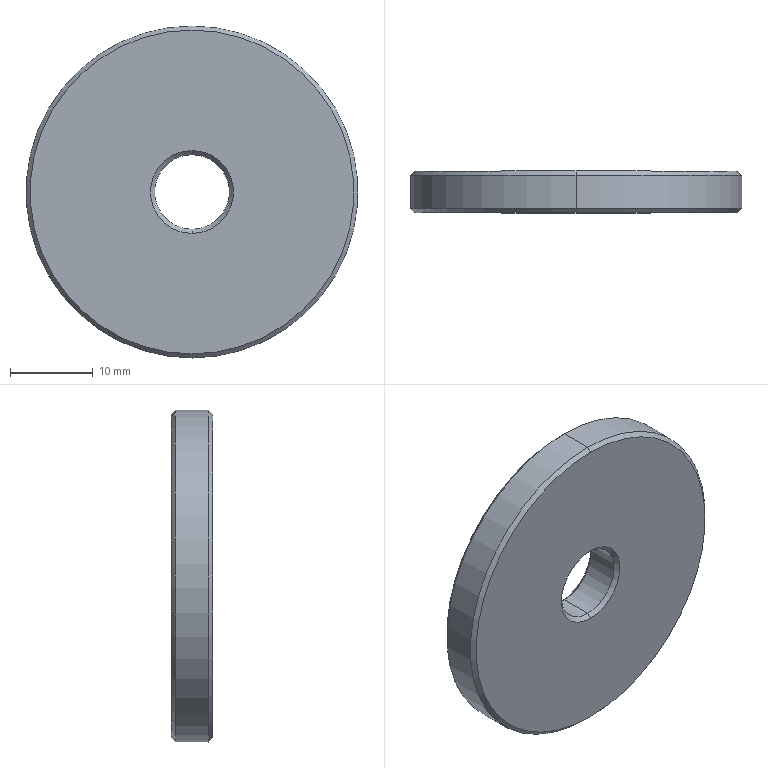Part | SolidWorks | features BaseBody 1 | 1 solid | 14 faces | box 40 x 5 x 40 mm | volume 5927 mm3 | cone 8 | cylinder 4 | plane 2 | commonest cylinder face diameters 9 x2 40 x2
STEP:
#1=CARTESIAN_POINT('',(0.,4.5,-4.5));
#2=VERTEX_POINT('',#1);
#3=CARTESIAN_POINT('',(0.,4.5,4.5));
#4=VERTEX_POINT('',#3);
#5=CARTESIAN_POINT('',(0.,4.5,0.));
#6=DIRECTION('',(0.,1.,0.));
#7=DIRECTION('',(0.,0.,-1.));
#8=AXIS2_PLACEMENT_3D('',#5,#6,#7);
#9=CIRCLE('',#8,4.5);
#10=EDGE_CURVE('',#2,#4,#9,.T.);
#11=ORIENTED_EDGE('',*,*,#10,.F.);
#12=CARTESIAN_POINT('',(0.,5.,-5.));
#13=VERTEX_POINT('',#12);
#14=CARTESIAN_POINT('',(0.,5.,-5.));
#15=DIRECTION('',(0.,0.7071,-0.7071));
#16=VECTOR('',#15,1000.);
#17=LINE('',#14,#16);
#18=EDGE_CURVE('',#2,#13,#17,.T.);
#19=ORIENTED_EDGE('',*,*,#18,.T.);
#20=CARTESIAN_POINT('',(0.,5.,5.));
#21=VERTEX_POINT('',#20);
#22=CARTESIAN_POINT('',(0.,5.,0.));
#23=DIRECTION('',(0.,-1.,0.));
#24=DIRECTION('',(0.,0.,1.));
#25=AXIS2_PLACEMENT_3D('',#22,#23,#24);
#26=CIRCLE('',#25,5.);
#27=EDGE_CURVE('',#21,#13,#26,.T.);
#28=ORIENTED_EDGE('',*,*,#27,.F.);
#29=CARTESIAN_POINT('',(0.,5.,5.));
#30=DIRECTION('',(0.,0.7071,0.7071));
#31=VECTOR('',#30,1000.);
#32=LINE('',#29,#31);
#33=EDGE_CURVE('',#4,#21,#32,.T.);
#34=ORIENTED_EDGE('',*,*,#33,.F.);
#35=EDGE_LOOP('',(#11,#19,#28,#34));
#36=FACE_OUTER_BOUND('',#35,.T.);
#37=CARTESIAN_POINT('',(0.,5.,0.));
#38=DIRECTION('',(0.,1.,0.));
#39=DIRECTION('',(0.,0.,1.));
#40=AXIS2_PLACEMENT_3D('',#37,#38,#39);
#41=CONICAL_SURFACE('',#40,5.,0.7854);
#42=ADVANCED_FACE('',(#36),#41,.F.);
#43=CARTESIAN_POINT('',(0.,5.,19.5));
#44=VERTEX_POINT('',#43);
#45=CARTESIAN_POINT('',(0.,5.,-19.5));
#46=VERTEX_POINT('',#45);
#47=CARTESIAN_POINT('',(0.,5.,0.));
#48=DIRECTION('',(0.,1.,0.));
#49=DIRECTION('',(0.,0.,-1.));
#50=AXIS2_PLACEMENT_3D('',#47,#48,#49);
#51=CIRCLE('',#50,19.5);
#52=EDGE_CURVE('',#44,#46,#51,.T.);
#53=ORIENTED_EDGE('',*,*,#52,.F.);
#54=CARTESIAN_POINT('',(0.,4.5,20.));
#55=VERTEX_POINT('',#54);
#56=CARTESIAN_POINT('',(0.,4.5,20.));
#57=DIRECTION('',(0.,-0.7071,0.7071));
#58=VECTOR('',#57,1000.);
#59=LINE('',#56,#58);
#60=EDGE_CURVE('',#44,#55,#59,.T.);
#61=ORIENTED_EDGE('',*,*,#60,.T.);
#62=CARTESIAN_POINT('',(0.,4.5,-20.));
#63=VERTEX_POINT('',#62);
#64=CARTESIAN_POINT('',(0.,4.5,0.));
#65=DIRECTION('',(0.,1.,0.));
#66=DIRECTION('',(0.,0.,-1.));
#67=AXIS2_PLACEMENT_3D('',#64,#65,#66);
#68=CIRCLE('',#67,20.);
#69=EDGE_CURVE('',#55,#63,#68,.T.);
#70=ORIENTED_EDGE('',*,*,#69,.T.);
#71=CARTESIAN_POINT('',(0.,4.5,-20.));
#72=DIRECTION('',(0.,-0.7071,-0.7071));
#73=VECTOR('',#72,1000.);
#74=LINE('',#71,#73);
#75=EDGE_CURVE('',#46,#63,#74,.T.);
#76=ORIENTED_EDGE('',*,*,#75,.F.);
#77=EDGE_LOOP('',(#53,#61,#70,#76));
#78=FACE_OUTER_BOUND('',#77,.T.);
#79=CARTESIAN_POINT('',(0.,4.5,0.));
#80=DIRECTION('',(0.,-1.,0.));
#81=DIRECTION('',(0.,0.,-1.));
#82=AXIS2_PLACEMENT_3D('',#79,#80,#81);
#83=CONICAL_SURFACE('',#82,20.,0.7854);
#84=ADVANCED_FACE('',(#78),#83,.T.);
#85=CARTESIAN_POINT('',(0.,0.5,-4.5));
#86=VERTEX_POINT('',#85);
#87=CARTESIAN_POINT('',(0.,0.5,4.5));
#88=VERTEX_POINT('',#87);
#89=CARTESIAN_POINT('',(0.,0.5,0.));
#90=DIRECTION('',(0.,1.,0.));
#91=DIRECTION('',(0.,0.,1.));
#92=AXIS2_PLACEMENT_3D('',#89,#90,#91);
#93=CIRCLE('',#92,4.5);
#94=EDGE_CURVE('',#86,#88,#93,.T.);
#95=ORIENTED_EDGE('',*,*,#94,.F.);
#96=CARTESIAN_POINT('',(0.,0.,-4.5));
#97=DIRECTION('',(0.,1.,0.));
#98=VECTOR('',#97,1000.);
#99=LINE('',#96,#98);
#100=EDGE_CURVE('',#86,#2,#99,.T.);
#101=ORIENTED_EDGE('',*,*,#100,.T.);
#102=ORIENTED_EDGE('',*,*,#10,.T.);
#103=CARTESIAN_POINT('',(0.,0.,4.5));
#104=DIRECTION('',(0.,1.,0.));
#105=VECTOR('',#104,1000.);
#106=LINE('',#103,#105);
#107=EDGE_CURVE('',#88,#4,#106,.T.);
#108=ORIENTED_EDGE('',*,*,#107,.F.);
#109=EDGE_LOOP('',(#95,#101,#102,#108));
#110=FACE_OUTER_BOUND('',#109,.T.);
#111=CARTESIAN_POINT('',(0.,0.,0.));
#112=DIRECTION('',(0.,1.,0.));
#113=DIRECTION('',(0.,0.,1.));
#114=AXIS2_PLACEMENT_3D('',#111,#112,#113);
#115=CYLINDRICAL_SURFACE('',#114,4.5);
#116=ADVANCED_FACE('',(#110),#115,.F.);
#117=CARTESIAN_POINT('',(0.,0.5,20.));
#118=VERTEX_POINT('',#117);
#119=CARTESIAN_POINT('',(0.,0.5,-20.));
#120=VERTEX_POINT('',#119);
#121=CARTESIAN_POINT('',(0.,0.5,0.));
#122=DIRECTION('',(0.,1.,0.));
#123=DIRECTION('',(0.,0.,1.));
#124=AXIS2_PLACEMENT_3D('',#121,#122,#123);
#125=CIRCLE('',#124,20.);
#126=EDGE_CURVE('',#118,#120,#125,.T.);
#127=ORIENTED_EDGE('',*,*,#126,.T.);
#128=CARTESIAN_POINT('',(0.,0.,-20.));
#129=DIRECTION('',(0.,1.,0.));
#130=VECTOR('',#129,1000.);
#131=LINE('',#128,#130);
#132=EDGE_CURVE('',#120,#63,#131,.T.);
#133=ORIENTED_EDGE('',*,*,#132,.T.);
#134=ORIENTED_EDGE('',*,*,#69,.F.);
#135=CARTESIAN_POINT('',(0.,0.,20.));
#136=DIRECTION('',(0.,1.,0.));
#137=VECTOR('',#136,1000.);
#138=LINE('',#135,#137);
#139=EDGE_CURVE('',#118,#55,#138,.T.);
#140=ORIENTED_EDGE('',*,*,#139,.F.);
#141=EDGE_LOOP('',(#127,#133,#134,#140));
#142=FACE_OUTER_BOUND('',#141,.T.);
#143=CARTESIAN_POINT('',(0.,0.,0.));
#144=DIRECTION('',(0.,1.,0.));
#145=DIRECTION('',(0.,0.,1.));
#146=AXIS2_PLACEMENT_3D('',#143,#144,#145);
#147=CYLINDRICAL_SURFACE('',#146,20.);
#148=ADVANCED_FACE('',(#142),#147,.T.);
#149=ORIENTED_EDGE('',*,*,#94,.T.);
#150=CARTESIAN_POINT('',(0.,0.,5.));
#151=VERTEX_POINT('',#150);
#152=CARTESIAN_POINT('',(0.,0.,5.));
#153=DIRECTION('',(0.,-0.7071,0.7071));
#154=VECTOR('',#153,1000.);
#155=LINE('',#152,#154);
#156=EDGE_CURVE('',#88,#151,#155,.T.);
#157=ORIENTED_EDGE('',*,*,#156,.T.);
#158=CARTESIAN_POINT('',(0.,0.,-5.));
#159=VERTEX_POINT('',#158);
#160=CARTESIAN_POINT('',(0.,0.,0.));
#161=DIRECTION('',(0.,1.,0.));
#162=DIRECTION('',(0.,0.,-1.));
#163=AXIS2_PLACEMENT_3D('',#160,#161,#162);
#164=CIRCLE('',#163,5.);
#165=EDGE_CURVE('',#159,#151,#164,.T.);
#166=ORIENTED_EDGE('',*,*,#165,.F.);
#167=CARTESIAN_POINT('',(0.,0.,-5.));
#168=DIRECTION('',(0.,-0.7071,-0.7071));
#169=VECTOR('',#168,1000.);
#170=LINE('',#167,#169);
#171=EDGE_CURVE('',#86,#159,#170,.T.);
#172=ORIENTED_EDGE('',*,*,#171,.F.);
#173=EDGE_LOOP('',(#149,#157,#166,#172));
#174=FACE_OUTER_BOUND('',#173,.T.);
#175=CARTESIAN_POINT('',(0.,0.,0.));
#176=DIRECTION('',(0.,-1.,0.));
#177=DIRECTION('',(0.,0.,-1.));
#178=AXIS2_PLACEMENT_3D('',#175,#176,#177);
#179=CONICAL_SURFACE('',#178,5.,0.7854);
#180=ADVANCED_FACE('',(#174),#179,.F.);
#181=CARTESIAN_POINT('',(0.,0.,19.5));
#182=VERTEX_POINT('',#181);
#183=CARTESIAN_POINT('',(0.,0.,-19.5));
#184=VERTEX_POINT('',#183);
#185=CARTESIAN_POINT('',(0.,0.,0.));
#186=DIRECTION('',(0.,1.,0.));
#187=DIRECTION('',(0.,0.,1.));
#188=AXIS2_PLACEMENT_3D('',#185,#186,#187);
#189=CIRCLE('',#188,19.5);
#190=EDGE_CURVE('',#182,#184,#189,.T.);
#191=ORIENTED_EDGE('',*,*,#190,.T.);
#192=CARTESIAN_POINT('',(0.,0.5,-20.));
#193=DIRECTION('',(0.,0.7071,-0.7071));
#194=VECTOR('',#193,1000.);
#195=LINE('',#192,#194);
#196=EDGE_CURVE('',#184,#120,#195,.T.);
#197=ORIENTED_EDGE('',*,*,#196,.T.);
#198=ORIENTED_EDGE('',*,*,#126,.F.);
#199=CARTESIAN_POINT('',(0.,0.5,20.));
#200=DIRECTION('',(0.,0.7071,0.7071));
#201=VECTOR('',#200,1000.);
#202=LINE('',#199,#201);
#203=EDGE_CURVE('',#182,#118,#202,.T.);
#204=ORIENTED_EDGE('',*,*,#203,.F.);
#205=EDGE_LOOP('',(#191,#197,#198,#204));
#206=FACE_OUTER_BOUND('',#205,.T.);
#207=CARTESIAN_POINT('',(0.,0.5,0.));
#208=DIRECTION('',(0.,1.,0.));
#209=DIRECTION('',(0.,0.,1.));
#210=AXIS2_PLACEMENT_3D('',#207,#208,#209);
#211=CONICAL_SURFACE('',#210,20.,0.7854);
#212=ADVANCED_FACE('',(#206),#211,.T.);
#213=ORIENTED_EDGE('',*,*,#27,.T.);
#214=CARTESIAN_POINT('',(0.,5.,0.));
#215=DIRECTION('',(0.,-1.,0.));
#216=DIRECTION('',(0.,0.,1.));
#217=AXIS2_PLACEMENT_3D('',#214,#215,#216);
#218=CIRCLE('',#217,5.);
#219=EDGE_CURVE('',#13,#21,#218,.T.);
#220=ORIENTED_EDGE('',*,*,#219,.T.);
#221=EDGE_LOOP('',(#213,#220));
#222=FACE_BOUND('',#221,.T.);
#223=CARTESIAN_POINT('',(0.,5.,0.));
#224=DIRECTION('',(0.,1.,0.));
#225=DIRECTION('',(0.,0.,-1.));
#226=AXIS2_PLACEMENT_3D('',#223,#224,#225);
#227=CIRCLE('',#226,19.5);
#228=EDGE_CURVE('',#46,#44,#227,.T.);
#229=ORIENTED_EDGE('',*,*,#228,.T.);
#230=ORIENTED_EDGE('',*,*,#52,.T.);
#231=EDGE_LOOP('',(#229,#230));
#232=FACE_OUTER_BOUND('',#231,.T.);
#233=CARTESIAN_POINT('',(0.,5.,0.));
#234=DIRECTION('',(0.,1.,0.));
#235=DIRECTION('',(0.,0.,1.));
#236=AXIS2_PLACEMENT_3D('',#233,#234,#235);
#237=PLANE('',#236);
#238=ADVANCED_FACE('',(#222,#232),#237,.T.);
#239=ORIENTED_EDGE('',*,*,#18,.F.);
#240=CARTESIAN_POINT('',(0.,4.5,0.));
#241=DIRECTION('',(0.,1.,0.));
#242=DIRECTION('',(0.,0.,-1.));
#243=AXIS2_PLACEMENT_3D('',#240,#241,#242);
#244=CIRCLE('',#243,4.5);
#245=EDGE_CURVE('',#4,#2,#244,.T.);
#246=ORIENTED_EDGE('',*,*,#245,.F.);
#247=ORIENTED_EDGE('',*,*,#33,.T.);
#248=ORIENTED_EDGE('',*,*,#219,.F.);
#249=EDGE_LOOP('',(#239,#246,#247,#248));
#250=FACE_OUTER_BOUND('',#249,.T.);
#251=CARTESIAN_POINT('',(0.,5.,0.));
#252=DIRECTION('',(0.,1.,0.));
#253=DIRECTION('',(0.,0.,1.));
#254=AXIS2_PLACEMENT_3D('',#251,#252,#253);
#255=CONICAL_SURFACE('',#254,5.,0.7854);
#256=ADVANCED_FACE('',(#250),#255,.F.);
#257=ORIENTED_EDGE('',*,*,#60,.F.);
#258=ORIENTED_EDGE('',*,*,#228,.F.);
#259=ORIENTED_EDGE('',*,*,#75,.T.);
#260=CARTESIAN_POINT('',(0.,4.5,0.));
#261=DIRECTION('',(0.,1.,0.));
#262=DIRECTION('',(0.,0.,-1.));
#263=AXIS2_PLACEMENT_3D('',#260,#261,#262);
#264=CIRCLE('',#263,20.);
#265=EDGE_CURVE('',#63,#55,#264,.T.);
#266=ORIENTED_EDGE('',*,*,#265,.T.);
#267=EDGE_LOOP('',(#257,#258,#259,#266));
#268=FACE_OUTER_BOUND('',#267,.T.);
#269=CARTESIAN_POINT('',(0.,4.5,0.));
#270=DIRECTION('',(0.,-1.,0.));
#271=DIRECTION('',(0.,0.,-1.));
#272=AXIS2_PLACEMENT_3D('',#269,#270,#271);
#273=CONICAL_SURFACE('',#272,20.,0.7854);
#274=ADVANCED_FACE('',(#268),#273,.T.);
#275=ORIENTED_EDGE('',*,*,#100,.F.);
#276=CARTESIAN_POINT('',(0.,0.5,0.));
#277=DIRECTION('',(0.,1.,0.));
#278=DIRECTION('',(0.,0.,1.));
#279=AXIS2_PLACEMENT_3D('',#276,#277,#278);
#280=CIRCLE('',#279,4.5);
#281=EDGE_CURVE('',#88,#86,#280,.T.);
#282=ORIENTED_EDGE('',*,*,#281,.F.);
#283=ORIENTED_EDGE('',*,*,#107,.T.);
#284=ORIENTED_EDGE('',*,*,#245,.T.);
#285=EDGE_LOOP('',(#275,#282,#283,#284));
#286=FACE_OUTER_BOUND('',#285,.T.);
#287=CARTESIAN_POINT('',(0.,0.,0.));
#288=DIRECTION('',(0.,1.,0.));
#289=DIRECTION('',(0.,0.,1.));
#290=AXIS2_PLACEMENT_3D('',#287,#288,#289);
#291=CYLINDRICAL_SURFACE('',#290,4.5);
#292=ADVANCED_FACE('',(#286),#291,.F.);
#293=ORIENTED_EDGE('',*,*,#132,.F.);
#294=CARTESIAN_POINT('',(0.,0.5,0.));
#295=DIRECTION('',(0.,1.,0.));
#296=DIRECTION('',(0.,0.,1.));
#297=AXIS2_PLACEMENT_3D('',#294,#295,#296);
#298=CIRCLE('',#297,20.);
#299=EDGE_CURVE('',#120,#118,#298,.T.);
#300=ORIENTED_EDGE('',*,*,#299,.T.);
#301=ORIENTED_EDGE('',*,*,#139,.T.);
#302=ORIENTED_EDGE('',*,*,#265,.F.);
#303=EDGE_LOOP('',(#293,#300,#301,#302));
#304=FACE_OUTER_BOUND('',#303,.T.);
#305=CARTESIAN_POINT('',(0.,0.,0.));
#306=DIRECTION('',(0.,1.,0.));
#307=DIRECTION('',(0.,0.,1.));
#308=AXIS2_PLACEMENT_3D('',#305,#306,#307);
#309=CYLINDRICAL_SURFACE('',#308,20.);
#310=ADVANCED_FACE('',(#304),#309,.T.);
#311=ORIENTED_EDGE('',*,*,#156,.F.);
#312=ORIENTED_EDGE('',*,*,#281,.T.);
#313=ORIENTED_EDGE('',*,*,#171,.T.);
#314=CARTESIAN_POINT('',(0.,0.,0.));
#315=DIRECTION('',(0.,1.,0.));
#316=DIRECTION('',(0.,0.,-1.));
#317=AXIS2_PLACEMENT_3D('',#314,#315,#316);
#318=CIRCLE('',#317,5.);
#319=EDGE_CURVE('',#151,#159,#318,.T.);
#320=ORIENTED_EDGE('',*,*,#319,.F.);
#321=EDGE_LOOP('',(#311,#312,#313,#320));
#322=FACE_OUTER_BOUND('',#321,.T.);
#323=CARTESIAN_POINT('',(0.,0.,0.));
#324=DIRECTION('',(0.,-1.,0.));
#325=DIRECTION('',(0.,0.,-1.));
#326=AXIS2_PLACEMENT_3D('',#323,#324,#325);
#327=CONICAL_SURFACE('',#326,5.,0.7854);
#328=ADVANCED_FACE('',(#322),#327,.F.);
#329=ORIENTED_EDGE('',*,*,#196,.F.);
#330=CARTESIAN_POINT('',(0.,0.,0.));
#331=DIRECTION('',(0.,1.,0.));
#332=DIRECTION('',(0.,0.,1.));
#333=AXIS2_PLACEMENT_3D('',#330,#331,#332);
#334=CIRCLE('',#333,19.5);
#335=EDGE_CURVE('',#184,#182,#334,.T.);
#336=ORIENTED_EDGE('',*,*,#335,.T.);
#337=ORIENTED_EDGE('',*,*,#203,.T.);
#338=ORIENTED_EDGE('',*,*,#299,.F.);
#339=EDGE_LOOP('',(#329,#336,#337,#338));
#340=FACE_OUTER_BOUND('',#339,.T.);
#341=CARTESIAN_POINT('',(0.,0.5,0.));
#342=DIRECTION('',(0.,1.,0.));
#343=DIRECTION('',(0.,0.,1.));
#344=AXIS2_PLACEMENT_3D('',#341,#342,#343);
#345=CONICAL_SURFACE('',#344,20.,0.7854);
#346=ADVANCED_FACE('',(#340),#345,.T.);
#347=ORIENTED_EDGE('',*,*,#165,.T.);
#348=ORIENTED_EDGE('',*,*,#319,.T.);
#349=EDGE_LOOP('',(#347,#348));
#350=FACE_BOUND('',#349,.T.);
#351=ORIENTED_EDGE('',*,*,#190,.F.);
#352=ORIENTED_EDGE('',*,*,#335,.F.);
#353=EDGE_LOOP('',(#351,#352));
#354=FACE_OUTER_BOUND('',#353,.T.);
#355=CARTESIAN_POINT('',(0.,0.,0.));
#356=DIRECTION('',(0.,1.,0.));
#357=DIRECTION('',(0.,0.,1.));
#358=AXIS2_PLACEMENT_3D('',#355,#356,#357);
#359=PLANE('',#358);
#360=ADVANCED_FACE('',(#350,#354),#359,.F.);
#361=CLOSED_SHELL('',(#42,#84,#116,#148,#180,#212,#238,#256,#274,#292,#310,#328,#346,#360));
#362=MANIFOLD_SOLID_BREP('',#361);
#363=CARTESIAN_POINT('',(0.,0.,0.));
#364=DIRECTION('',(0.,0.,1.));
#365=DIRECTION('',(1.,0.,0.));
#366=AXIS2_PLACEMENT_3D('',#363,#364,#365);
#367=(LENGTH_UNIT()NAMED_UNIT(*)SI_UNIT(.MILLI.,.METRE.));
#368=UNCERTAINTY_MEASURE_WITH_UNIT(LENGTH_MEASURE(0.00001),#367,'','');
#369=(NAMED_UNIT(*)PLANE_ANGLE_UNIT()SI_UNIT($,.RADIAN.));
#370=(NAMED_UNIT(*)SI_UNIT($,.STERADIAN.)SOLID_ANGLE_UNIT());
#371=(GEOMETRIC_REPRESENTATION_CONTEXT(3)GLOBAL_UNCERTAINTY_ASSIGNED_CONTEXT((#368))GLOBAL_UNIT_ASSIGNED_CONTEXT((#367,#369,#370))REPRESENTATION_CONTEXT('',''));
#372=ADVANCED_BREP_SHAPE_REPRESENTATION('',(#362,#366),#371);